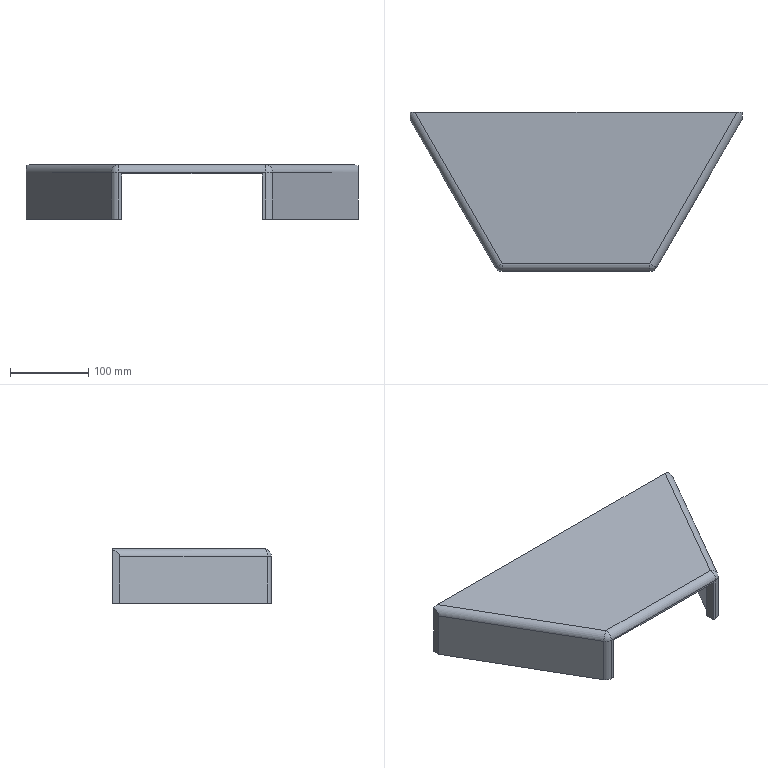Part | SolidWorks | features ICE 4, Fillet 2, Extrusion 1, Shell 1 | 1 solid | 25 faces | box 424 x 203 x 70 mm | volume 1081632 mm3 | plane 18 | cylinder 5 | sphere 2 | commonest cylinder face diameters 20 x5
STEP:
#1=CARTESIAN_POINT('',(90.,-95.5,58.));
#2=VERTEX_POINT('',#1);
#3=CARTESIAN_POINT('',(90.,-95.5,0.));
#4=VERTEX_POINT('',#3);
#5=CARTESIAN_POINT('',(90.,-95.5,70.));
#6=DIRECTION('',(0.,0.,-1.));
#7=VECTOR('',#6,1000.);
#8=LINE('',#5,#7);
#9=EDGE_CURVE('',#2,#4,#8,.T.);
#10=ORIENTED_EDGE('',*,*,#9,.F.);
#11=CARTESIAN_POINT('',(93.072,-95.5,58.));
#12=VERTEX_POINT('',#11);
#13=CARTESIAN_POINT('',(-93.072,-95.5,58.));
#14=DIRECTION('',(1.,0.,0.));
#15=VECTOR('',#14,1000.);
#16=LINE('',#13,#15);
#17=EDGE_CURVE('',#2,#12,#16,.T.);
#18=ORIENTED_EDGE('',*,*,#17,.T.);
#19=CARTESIAN_POINT('',(93.072,-95.5,0.));
#20=VERTEX_POINT('',#19);
#21=CARTESIAN_POINT('',(93.072,-95.5,70.));
#22=DIRECTION('',(0.,0.,-1.));
#23=VECTOR('',#22,1000.);
#24=LINE('',#21,#23);
#25=EDGE_CURVE('',#12,#20,#24,.T.);
#26=ORIENTED_EDGE('',*,*,#25,.T.);
#27=CARTESIAN_POINT('',(0.,-95.5,0.));
#28=DIRECTION('',(1.,0.,0.));
#29=VECTOR('',#28,1000.);
#30=LINE('',#27,#29);
#31=EDGE_CURVE('',#4,#20,#30,.T.);
#32=ORIENTED_EDGE('',*,*,#31,.F.);
#33=EDGE_LOOP('',(#10,#18,#26,#32));
#34=FACE_OUTER_BOUND('',#33,.T.);
#35=CARTESIAN_POINT('',(212.,-95.5,70.));
#36=DIRECTION('',(0.,1.,0.));
#37=DIRECTION('',(-1.,0.,0.));
#38=AXIS2_PLACEMENT_3D('',#35,#36,#37);
#39=PLANE('',#38);
#40=ADVANCED_FACE('',(#34),#39,.T.);
#41=CARTESIAN_POINT('',(212.,86.49,0.));
#42=VERTEX_POINT('',#41);
#43=CARTESIAN_POINT('',(102.887,-102.5,0.));
#44=VERTEX_POINT('',#43);
#45=CARTESIAN_POINT('',(121.549,-70.176,0.));
#46=DIRECTION('',(-0.5,-0.866,0.));
#47=VECTOR('',#46,1000.);
#48=LINE('',#45,#47);
#49=EDGE_CURVE('',#42,#44,#48,.T.);
#50=ORIENTED_EDGE('',*,*,#49,.T.);
#51=CARTESIAN_POINT('',(94.226,-107.5,0.));
#52=VERTEX_POINT('',#51);
#53=CARTESIAN_POINT('',(94.226,-97.5,0.));
#54=DIRECTION('',(0.,0.,-1.));
#55=DIRECTION('',(-1.,0.,0.));
#56=AXIS2_PLACEMENT_3D('',#53,#54,#55);
#57=CIRCLE('',#56,10.);
#58=EDGE_CURVE('',#44,#52,#57,.T.);
#59=ORIENTED_EDGE('',*,*,#58,.T.);
#60=CARTESIAN_POINT('',(90.,-107.5,0.));
#61=VERTEX_POINT('',#60);
#62=CARTESIAN_POINT('',(212.,-107.5,0.));
#63=DIRECTION('',(1.,0.,0.));
#64=VECTOR('',#63,1000.);
#65=LINE('',#62,#64);
#66=EDGE_CURVE('',#61,#52,#65,.T.);
#67=ORIENTED_EDGE('',*,*,#66,.F.);
#68=CARTESIAN_POINT('',(90.,0.,0.));
#69=DIRECTION('',(0.,-1.,0.));
#70=VECTOR('',#69,1000.);
#71=LINE('',#68,#70);
#72=EDGE_CURVE('',#4,#61,#71,.T.);
#73=ORIENTED_EDGE('',*,*,#72,.F.);
#74=ORIENTED_EDGE('',*,*,#31,.T.);
#75=CARTESIAN_POINT('',(200.,89.705,0.));
#76=VERTEX_POINT('',#75);
#77=CARTESIAN_POINT('',(111.157,-64.176,0.));
#78=DIRECTION('',(-0.5,-0.866,0.));
#79=VECTOR('',#78,1000.);
#80=LINE('',#77,#79);
#81=EDGE_CURVE('',#76,#20,#80,.T.);
#82=ORIENTED_EDGE('',*,*,#81,.F.);
#83=CARTESIAN_POINT('',(200.,95.5,0.));
#84=VERTEX_POINT('',#83);
#85=CARTESIAN_POINT('',(200.,0.,0.));
#86=DIRECTION('',(0.,1.,0.));
#87=VECTOR('',#86,1000.);
#88=LINE('',#85,#87);
#89=EDGE_CURVE('',#76,#84,#88,.T.);
#90=ORIENTED_EDGE('',*,*,#89,.T.);
#91=CARTESIAN_POINT('',(212.,95.5,0.));
#92=VERTEX_POINT('',#91);
#93=CARTESIAN_POINT('',(-212.,95.5,0.));
#94=DIRECTION('',(-1.,0.,0.));
#95=VECTOR('',#94,1000.);
#96=LINE('',#93,#95);
#97=EDGE_CURVE('',#92,#84,#96,.T.);
#98=ORIENTED_EDGE('',*,*,#97,.F.);
#99=CARTESIAN_POINT('',(212.,107.5,0.));
#100=DIRECTION('',(0.,1.,0.));
#101=VECTOR('',#100,1000.);
#102=LINE('',#99,#101);
#103=EDGE_CURVE('',#42,#92,#102,.T.);
#104=ORIENTED_EDGE('',*,*,#103,.F.);
#105=EDGE_LOOP('',(#50,#59,#67,#73,#74,#82,#90,#98,#104));
#106=FACE_OUTER_BOUND('',#105,.T.);
#107=CARTESIAN_POINT('',(0.,0.,0.));
#108=DIRECTION('',(0.,0.,-1.));
#109=DIRECTION('',(-1.,0.,0.));
#110=AXIS2_PLACEMENT_3D('',#107,#108,#109);
#111=PLANE('',#110);
#112=ADVANCED_FACE('',(#106),#111,.T.);
#113=CARTESIAN_POINT('',(-200.,95.5,58.));
#114=VERTEX_POINT('',#113);
#115=CARTESIAN_POINT('',(-200.,95.5,0.));
#116=VERTEX_POINT('',#115);
#117=CARTESIAN_POINT('',(-200.,95.5,70.));
#118=DIRECTION('',(0.,0.,-1.));
#119=VECTOR('',#118,1000.);
#120=LINE('',#117,#119);
#121=EDGE_CURVE('',#114,#116,#120,.T.);
#122=ORIENTED_EDGE('',*,*,#121,.F.);
#123=CARTESIAN_POINT('',(-200.,89.705,58.));
#124=VERTEX_POINT('',#123);
#125=CARTESIAN_POINT('',(-200.,89.705,58.));
#126=DIRECTION('',(0.,-1.,0.));
#127=VECTOR('',#126,1000.);
#128=LINE('',#125,#127);
#129=EDGE_CURVE('',#114,#124,#128,.T.);
#130=ORIENTED_EDGE('',*,*,#129,.T.);
#131=CARTESIAN_POINT('',(-200.,89.705,0.));
#132=VERTEX_POINT('',#131);
#133=CARTESIAN_POINT('',(-200.,89.705,70.));
#134=DIRECTION('',(0.,0.,-1.));
#135=VECTOR('',#134,1000.);
#136=LINE('',#133,#135);
#137=EDGE_CURVE('',#124,#132,#136,.T.);
#138=ORIENTED_EDGE('',*,*,#137,.T.);
#139=CARTESIAN_POINT('',(-200.,0.,0.));
#140=DIRECTION('',(0.,-1.,0.));
#141=VECTOR('',#140,1000.);
#142=LINE('',#139,#141);
#143=EDGE_CURVE('',#116,#132,#142,.T.);
#144=ORIENTED_EDGE('',*,*,#143,.F.);
#145=EDGE_LOOP('',(#122,#130,#138,#144));
#146=FACE_OUTER_BOUND('',#145,.T.);
#147=CARTESIAN_POINT('',(-200.,107.5,70.));
#148=DIRECTION('',(1.,0.,0.));
#149=DIRECTION('',(0.,1.,0.));
#150=AXIS2_PLACEMENT_3D('',#147,#148,#149);
#151=PLANE('',#150);
#152=ADVANCED_FACE('',(#146),#151,.T.);
#153=CARTESIAN_POINT('',(-90.,-95.5,0.));
#154=VERTEX_POINT('',#153);
#155=CARTESIAN_POINT('',(-90.,-95.5,58.));
#156=VERTEX_POINT('',#155);
#157=CARTESIAN_POINT('',(-90.,-95.5,70.));
#158=DIRECTION('',(0.,0.,1.));
#159=VECTOR('',#158,1000.);
#160=LINE('',#157,#159);
#161=EDGE_CURVE('',#154,#156,#160,.T.);
#162=ORIENTED_EDGE('',*,*,#161,.F.);
#163=CARTESIAN_POINT('',(-93.072,-95.5,0.));
#164=VERTEX_POINT('',#163);
#165=CARTESIAN_POINT('',(0.,-95.5,0.));
#166=DIRECTION('',(1.,0.,0.));
#167=VECTOR('',#166,1000.);
#168=LINE('',#165,#167);
#169=EDGE_CURVE('',#164,#154,#168,.T.);
#170=ORIENTED_EDGE('',*,*,#169,.F.);
#171=CARTESIAN_POINT('',(-93.072,-95.5,58.));
#172=VERTEX_POINT('',#171);
#173=CARTESIAN_POINT('',(-93.072,-95.5,70.));
#174=DIRECTION('',(0.,0.,-1.));
#175=VECTOR('',#174,1000.);
#176=LINE('',#173,#175);
#177=EDGE_CURVE('',#172,#164,#176,.T.);
#178=ORIENTED_EDGE('',*,*,#177,.F.);
#179=CARTESIAN_POINT('',(-93.072,-95.5,58.));
#180=DIRECTION('',(1.,0.,0.));
#181=VECTOR('',#180,1000.);
#182=LINE('',#179,#181);
#183=EDGE_CURVE('',#172,#156,#182,.T.);
#184=ORIENTED_EDGE('',*,*,#183,.T.);
#185=EDGE_LOOP('',(#162,#170,#178,#184));
#186=FACE_OUTER_BOUND('',#185,.T.);
#187=CARTESIAN_POINT('',(212.,-95.5,70.));
#188=DIRECTION('',(0.,1.,0.));
#189=DIRECTION('',(-1.,0.,0.));
#190=AXIS2_PLACEMENT_3D('',#187,#188,#189);
#191=PLANE('',#190);
#192=ADVANCED_FACE('',(#186),#191,.T.);
#193=CARTESIAN_POINT('',(200.,89.705,58.));
#194=VERTEX_POINT('',#193);
#195=CARTESIAN_POINT('',(200.,89.705,70.));
#196=DIRECTION('',(0.,0.,1.));
#197=VECTOR('',#196,1000.);
#198=LINE('',#195,#197);
#199=EDGE_CURVE('',#76,#194,#198,.T.);
#200=ORIENTED_EDGE('',*,*,#199,.T.);
#201=CARTESIAN_POINT('',(200.,95.5,58.));
#202=VERTEX_POINT('',#201);
#203=CARTESIAN_POINT('',(200.,89.705,58.));
#204=DIRECTION('',(0.,1.,0.));
#205=VECTOR('',#204,1000.);
#206=LINE('',#203,#205);
#207=EDGE_CURVE('',#194,#202,#206,.T.);
#208=ORIENTED_EDGE('',*,*,#207,.T.);
#209=CARTESIAN_POINT('',(200.,95.5,70.));
#210=DIRECTION('',(0.,0.,-1.));
#211=VECTOR('',#210,1000.);
#212=LINE('',#209,#211);
#213=EDGE_CURVE('',#202,#84,#212,.T.);
#214=ORIENTED_EDGE('',*,*,#213,.T.);
#215=ORIENTED_EDGE('',*,*,#89,.F.);
#216=EDGE_LOOP('',(#200,#208,#214,#215));
#217=FACE_OUTER_BOUND('',#216,.T.);
#218=CARTESIAN_POINT('',(200.,107.5,70.));
#219=DIRECTION('',(-1.,0.,0.));
#220=DIRECTION('',(0.,-1.,0.));
#221=AXIS2_PLACEMENT_3D('',#218,#219,#220);
#222=PLANE('',#221);
#223=ADVANCED_FACE('',(#217),#222,.T.);
#224=CARTESIAN_POINT('',(200.,89.705,58.));
#225=DIRECTION('',(0.5,0.866,0.));
#226=VECTOR('',#225,1000.);
#227=LINE('',#224,#226);
#228=EDGE_CURVE('',#12,#194,#227,.T.);
#229=ORIENTED_EDGE('',*,*,#228,.T.);
#230=ORIENTED_EDGE('',*,*,#199,.F.);
#231=ORIENTED_EDGE('',*,*,#81,.T.);
#232=ORIENTED_EDGE('',*,*,#25,.F.);
#233=EDGE_LOOP('',(#229,#230,#231,#232));
#234=FACE_OUTER_BOUND('',#233,.T.);
#235=CARTESIAN_POINT('',(89.608,-101.5,70.));
#236=DIRECTION('',(0.866,-0.5,0.));
#237=DIRECTION('',(0.5,0.866,0.));
#238=AXIS2_PLACEMENT_3D('',#235,#236,#237);
#239=PLANE('',#238);
#240=ADVANCED_FACE('',(#234),#239,.F.);
#241=CARTESIAN_POINT('',(-93.072,-95.5,58.));
#242=DIRECTION('',(0.5,-0.866,0.));
#243=VECTOR('',#242,1000.);
#244=LINE('',#241,#243);
#245=EDGE_CURVE('',#124,#172,#244,.T.);
#246=ORIENTED_EDGE('',*,*,#245,.T.);
#247=ORIENTED_EDGE('',*,*,#177,.T.);
#248=CARTESIAN_POINT('',(-111.157,-64.176,0.));
#249=DIRECTION('',(-0.5,0.866,0.));
#250=VECTOR('',#249,1000.);
#251=LINE('',#248,#250);
#252=EDGE_CURVE('',#164,#132,#251,.T.);
#253=ORIENTED_EDGE('',*,*,#252,.T.);
#254=ORIENTED_EDGE('',*,*,#137,.F.);
#255=EDGE_LOOP('',(#246,#247,#253,#254));
#256=FACE_OUTER_BOUND('',#255,.T.);
#257=CARTESIAN_POINT('',(-213.738,113.5,70.));
#258=DIRECTION('',(-0.866,-0.5,0.));
#259=DIRECTION('',(0.5,-0.866,0.));
#260=AXIS2_PLACEMENT_3D('',#257,#258,#259);
#261=PLANE('',#260);
#262=ADVANCED_FACE('',(#256),#261,.F.);
#263=CARTESIAN_POINT('',(-94.226,-107.5,0.));
#264=VERTEX_POINT('',#263);
#265=CARTESIAN_POINT('',(-90.,-107.5,0.));
#266=VERTEX_POINT('',#265);
#267=CARTESIAN_POINT('',(212.,-107.5,0.));
#268=DIRECTION('',(1.,0.,0.));
#269=VECTOR('',#268,1000.);
#270=LINE('',#267,#269);
#271=EDGE_CURVE('',#264,#266,#270,.T.);
#272=ORIENTED_EDGE('',*,*,#271,.F.);
#273=CARTESIAN_POINT('',(-102.887,-102.5,0.));
#274=VERTEX_POINT('',#273);
#275=CARTESIAN_POINT('',(-94.226,-97.5,0.));
#276=DIRECTION('',(0.,0.,-1.));
#277=DIRECTION('',(-1.,0.,0.));
#278=AXIS2_PLACEMENT_3D('',#275,#276,#277);
#279=CIRCLE('',#278,10.);
#280=EDGE_CURVE('',#264,#274,#279,.T.);
#281=ORIENTED_EDGE('',*,*,#280,.T.);
#282=CARTESIAN_POINT('',(-212.,86.49,0.));
#283=VERTEX_POINT('',#282);
#284=CARTESIAN_POINT('',(-224.13,107.5,0.));
#285=DIRECTION('',(-0.5,0.866,0.));
#286=VECTOR('',#285,1000.);
#287=LINE('',#284,#286);
#288=EDGE_CURVE('',#274,#283,#287,.T.);
#289=ORIENTED_EDGE('',*,*,#288,.T.);
#290=CARTESIAN_POINT('',(-212.,95.5,0.));
#291=VERTEX_POINT('',#290);
#292=CARTESIAN_POINT('',(-212.,107.5,0.));
#293=DIRECTION('',(0.,-1.,0.));
#294=VECTOR('',#293,1000.);
#295=LINE('',#292,#294);
#296=EDGE_CURVE('',#291,#283,#295,.T.);
#297=ORIENTED_EDGE('',*,*,#296,.F.);
#298=CARTESIAN_POINT('',(-212.,95.5,0.));
#299=DIRECTION('',(-1.,0.,0.));
#300=VECTOR('',#299,1000.);
#301=LINE('',#298,#300);
#302=EDGE_CURVE('',#116,#291,#301,.T.);
#303=ORIENTED_EDGE('',*,*,#302,.F.);
#304=ORIENTED_EDGE('',*,*,#143,.T.);
#305=ORIENTED_EDGE('',*,*,#252,.F.);
#306=ORIENTED_EDGE('',*,*,#169,.T.);
#307=CARTESIAN_POINT('',(-90.,0.,0.));
#308=DIRECTION('',(0.,1.,0.));
#309=VECTOR('',#308,1000.);
#310=LINE('',#307,#309);
#311=EDGE_CURVE('',#266,#154,#310,.T.);
#312=ORIENTED_EDGE('',*,*,#311,.F.);
#313=EDGE_LOOP('',(#272,#281,#289,#297,#303,#304,#305,#306,#312));
#314=FACE_OUTER_BOUND('',#313,.T.);
#315=CARTESIAN_POINT('',(0.,0.,0.));
#316=DIRECTION('',(0.,0.,-1.));
#317=DIRECTION('',(-1.,0.,0.));
#318=AXIS2_PLACEMENT_3D('',#315,#316,#317);
#319=PLANE('',#318);
#320=ADVANCED_FACE('',(#314),#319,.T.);
#321=CARTESIAN_POINT('',(-212.,86.49,60.));
#322=VERTEX_POINT('',#321);
#323=CARTESIAN_POINT('',(-212.,86.49,70.));
#324=DIRECTION('',(0.,0.,-1.));
#325=VECTOR('',#324,1000.);
#326=LINE('',#323,#325);
#327=EDGE_CURVE('',#322,#283,#326,.T.);
#328=ORIENTED_EDGE('',*,*,#327,.F.);
#329=CARTESIAN_POINT('',(-212.,95.5,68.355));
#330=VERTEX_POINT('',#329);
#331=CARTESIAN_POINT('',(-212.,86.49,60.));
#332=CARTESIAN_POINT('',(-212.,86.49,63.439));
#333=CARTESIAN_POINT('',(-212.,89.754,66.466));
#334=CARTESIAN_POINT('',(-212.,95.5,68.355));
#335=(BOUNDED_CURVE()B_SPLINE_CURVE(3,(#331,#332,#333,#334),.UNSPECIFIED.,.F.,.F.)B_SPLINE_CURVE_WITH_KNOTS((4,4),(0.,0.989),.UNSPECIFIED.)CURVE()GEOMETRIC_REPRESENTATION_ITEM()RATIONAL_B_SPLINE_CURVE((1.,0.9201,0.9201,1.))REPRESENTATION_ITEM(''));
#336=EDGE_CURVE('',#322,#330,#335,.T.);
#337=ORIENTED_EDGE('',*,*,#336,.T.);
#338=CARTESIAN_POINT('',(-212.,95.5,70.));
#339=DIRECTION('',(0.,0.,-1.));
#340=VECTOR('',#339,1000.);
#341=LINE('',#338,#340);
#342=EDGE_CURVE('',#330,#291,#341,.T.);
#343=ORIENTED_EDGE('',*,*,#342,.T.);
#344=ORIENTED_EDGE('',*,*,#296,.T.);
#345=EDGE_LOOP('',(#328,#337,#343,#344));
#346=FACE_OUTER_BOUND('',#345,.T.);
#347=CARTESIAN_POINT('',(-212.,107.5,70.));
#348=DIRECTION('',(1.,0.,0.));
#349=DIRECTION('',(0.,1.,0.));
#350=AXIS2_PLACEMENT_3D('',#347,#348,#349);
#351=PLANE('',#350);
#352=ADVANCED_FACE('',(#346),#351,.F.);
#353=CARTESIAN_POINT('',(94.226,-107.5,60.));
#354=VERTEX_POINT('',#353);
#355=CARTESIAN_POINT('',(-94.226,-107.5,60.));
#356=VERTEX_POINT('',#355);
#357=CARTESIAN_POINT('',(212.,-107.5,60.));
#358=DIRECTION('',(-1.,0.,0.));
#359=VECTOR('',#358,1000.);
#360=LINE('',#357,#359);
#361=EDGE_CURVE('',#354,#356,#360,.T.);
#362=ORIENTED_EDGE('',*,*,#361,.T.);
#363=CARTESIAN_POINT('',(-94.226,-107.5,0.));
#364=DIRECTION('',(0.,0.,-1.));
#365=VECTOR('',#364,1000.);
#366=LINE('',#363,#365);
#367=EDGE_CURVE('',#356,#264,#366,.T.);
#368=ORIENTED_EDGE('',*,*,#367,.T.);
#369=ORIENTED_EDGE('',*,*,#271,.T.);
#370=CARTESIAN_POINT('',(-90.,-107.5,58.));
#371=VERTEX_POINT('',#370);
#372=CARTESIAN_POINT('',(-90.,-107.5,-74.019));
#373=DIRECTION('',(0.,0.,-1.));
#374=VECTOR('',#373,1000.);
#375=LINE('',#372,#374);
#376=EDGE_CURVE('',#371,#266,#375,.T.);
#377=ORIENTED_EDGE('',*,*,#376,.F.);
#378=CARTESIAN_POINT('',(90.,-107.5,58.));
#379=VERTEX_POINT('',#378);
#380=CARTESIAN_POINT('',(-90.,-107.5,58.));
#381=DIRECTION('',(-1.,0.,0.));
#382=VECTOR('',#381,1000.);
#383=LINE('',#380,#382);
#384=EDGE_CURVE('',#379,#371,#383,.T.);
#385=ORIENTED_EDGE('',*,*,#384,.F.);
#386=CARTESIAN_POINT('',(90.,-107.5,-74.019));
#387=DIRECTION('',(0.,0.,1.));
#388=VECTOR('',#387,1000.);
#389=LINE('',#386,#388);
#390=EDGE_CURVE('',#61,#379,#389,.T.);
#391=ORIENTED_EDGE('',*,*,#390,.F.);
#392=ORIENTED_EDGE('',*,*,#66,.T.);
#393=CARTESIAN_POINT('',(94.226,-107.5,70.));
#394=DIRECTION('',(0.,0.,1.));
#395=VECTOR('',#394,1000.);
#396=LINE('',#393,#395);
#397=EDGE_CURVE('',#52,#354,#396,.T.);
#398=ORIENTED_EDGE('',*,*,#397,.T.);
#399=EDGE_LOOP('',(#362,#368,#369,#377,#385,#391,#392,#398));
#400=FACE_OUTER_BOUND('',#399,.T.);
#401=CARTESIAN_POINT('',(212.,-107.5,70.));
#402=DIRECTION('',(0.,1.,0.));
#403=DIRECTION('',(-1.,0.,0.));
#404=AXIS2_PLACEMENT_3D('',#401,#402,#403);
#405=PLANE('',#404);
#406=ADVANCED_FACE('',(#400),#405,.F.);
#407=CARTESIAN_POINT('',(212.,95.5,68.355));
#408=VERTEX_POINT('',#407);
#409=CARTESIAN_POINT('',(212.,95.5,70.));
#410=DIRECTION('',(0.,0.,1.));
#411=VECTOR('',#410,1000.);
#412=LINE('',#409,#411);
#413=EDGE_CURVE('',#92,#408,#412,.T.);
#414=ORIENTED_EDGE('',*,*,#413,.T.);
#415=CARTESIAN_POINT('',(212.,86.49,60.));
#416=VERTEX_POINT('',#415);
#417=CARTESIAN_POINT('',(212.,95.5,68.355));
#418=CARTESIAN_POINT('',(212.,89.754,66.466));
#419=CARTESIAN_POINT('',(212.,86.49,63.439));
#420=CARTESIAN_POINT('',(212.,86.49,60.));
#421=(BOUNDED_CURVE()B_SPLINE_CURVE(3,(#417,#418,#419,#420),.UNSPECIFIED.,.F.,.T.)B_SPLINE_CURVE_WITH_KNOTS((4,4),(2.153,3.142),.UNSPECIFIED.)CURVE()GEOMETRIC_REPRESENTATION_ITEM()RATIONAL_B_SPLINE_CURVE((1.,0.9201,0.9201,1.))REPRESENTATION_ITEM(''));
#422=EDGE_CURVE('',#408,#416,#421,.T.);
#423=ORIENTED_EDGE('',*,*,#422,.T.);
#424=CARTESIAN_POINT('',(212.,86.49,70.));
#425=DIRECTION('',(0.,0.,1.));
#426=VECTOR('',#425,1000.);
#427=LINE('',#424,#426);
#428=EDGE_CURVE('',#42,#416,#427,.T.);
#429=ORIENTED_EDGE('',*,*,#428,.F.);
#430=ORIENTED_EDGE('',*,*,#103,.T.);
#431=EDGE_LOOP('',(#414,#423,#429,#430));
#432=FACE_OUTER_BOUND('',#431,.T.);
#433=CARTESIAN_POINT('',(212.,107.5,70.));
#434=DIRECTION('',(-1.,0.,0.));
#435=DIRECTION('',(0.,-1.,0.));
#436=AXIS2_PLACEMENT_3D('',#433,#434,#435);
#437=PLANE('',#436);
#438=ADVANCED_FACE('',(#432),#437,.F.);
#439=CARTESIAN_POINT('',(-94.226,-97.5,70.));
#440=VERTEX_POINT('',#439);
#441=CARTESIAN_POINT('',(94.226,-97.5,70.));
#442=VERTEX_POINT('',#441);
#443=CARTESIAN_POINT('',(0.,-97.5,70.));
#444=DIRECTION('',(1.,0.,0.));
#445=VECTOR('',#444,1000.);
#446=LINE('',#443,#445);
#447=EDGE_CURVE('',#440,#442,#446,.T.);
#448=ORIENTED_EDGE('',*,*,#447,.T.);
#449=CARTESIAN_POINT('',(205.655,95.5,70.));
#450=VERTEX_POINT('',#449);
#451=CARTESIAN_POINT('',(203.34,91.49,70.));
#452=DIRECTION('',(0.5,0.866,0.));
#453=VECTOR('',#452,1000.);
#454=LINE('',#451,#453);
#455=EDGE_CURVE('',#442,#450,#454,.T.);
#456=ORIENTED_EDGE('',*,*,#455,.T.);
#457=CARTESIAN_POINT('',(-205.655,95.5,70.));
#458=VERTEX_POINT('',#457);
#459=CARTESIAN_POINT('',(-212.,95.5,70.));
#460=DIRECTION('',(-1.,0.,0.));
#461=VECTOR('',#460,1000.);
#462=LINE('',#459,#461);
#463=EDGE_CURVE('',#450,#458,#462,.T.);
#464=ORIENTED_EDGE('',*,*,#463,.T.);
#465=CARTESIAN_POINT('',(-97.113,-92.5,70.));
#466=DIRECTION('',(0.5,-0.866,0.));
#467=VECTOR('',#466,1000.);
#468=LINE('',#465,#467);
#469=EDGE_CURVE('',#458,#440,#468,.T.);
#470=ORIENTED_EDGE('',*,*,#469,.T.);
#471=EDGE_LOOP('',(#448,#456,#464,#470));
#472=FACE_OUTER_BOUND('',#471,.T.);
#473=CARTESIAN_POINT('',(0.,0.,70.));
#474=DIRECTION('',(0.,0.,-1.));
#475=DIRECTION('',(-1.,0.,0.));
#476=AXIS2_PLACEMENT_3D('',#473,#474,#475);
#477=PLANE('',#476);
#478=ADVANCED_FACE('',(#472),#477,.F.);
#479=ORIENTED_EDGE('',*,*,#428,.T.);
#480=CARTESIAN_POINT('',(102.887,-102.5,60.));
#481=VERTEX_POINT('',#480);
#482=CARTESIAN_POINT('',(105.774,-97.5,60.));
#483=DIRECTION('',(-0.5,-0.866,0.));
#484=VECTOR('',#483,1000.);
#485=LINE('',#482,#484);
#486=EDGE_CURVE('',#416,#481,#485,.T.);
#487=ORIENTED_EDGE('',*,*,#486,.T.);
#488=CARTESIAN_POINT('',(102.887,-102.5,0.));
#489=DIRECTION('',(0.,0.,-1.));
#490=VECTOR('',#489,1000.);
#491=LINE('',#488,#490);
#492=EDGE_CURVE('',#481,#44,#491,.T.);
#493=ORIENTED_EDGE('',*,*,#492,.T.);
#494=ORIENTED_EDGE('',*,*,#49,.F.);
#495=EDGE_LOOP('',(#479,#487,#493,#494));
#496=FACE_OUTER_BOUND('',#495,.T.);
#497=CARTESIAN_POINT('',(100.,-107.5,70.));
#498=DIRECTION('',(0.866,-0.5,0.));
#499=DIRECTION('',(0.5,0.866,0.));
#500=AXIS2_PLACEMENT_3D('',#497,#498,#499);
#501=PLANE('',#500);
#502=ADVANCED_FACE('',(#496),#501,.T.);
#503=CARTESIAN_POINT('',(-102.887,-102.5,60.));
#504=VERTEX_POINT('',#503);
#505=CARTESIAN_POINT('',(-102.887,-102.5,70.));
#506=DIRECTION('',(0.,0.,1.));
#507=VECTOR('',#506,1000.);
#508=LINE('',#505,#507);
#509=EDGE_CURVE('',#274,#504,#508,.T.);
#510=ORIENTED_EDGE('',*,*,#509,.T.);
#511=CARTESIAN_POINT('',(-212.,86.49,60.));
#512=DIRECTION('',(-0.5,0.866,0.));
#513=VECTOR('',#512,1000.);
#514=LINE('',#511,#513);
#515=EDGE_CURVE('',#504,#322,#514,.T.);
#516=ORIENTED_EDGE('',*,*,#515,.T.);
#517=ORIENTED_EDGE('',*,*,#327,.T.);
#518=ORIENTED_EDGE('',*,*,#288,.F.);
#519=EDGE_LOOP('',(#510,#516,#517,#518));
#520=FACE_OUTER_BOUND('',#519,.T.);
#521=CARTESIAN_POINT('',(-224.13,107.5,70.));
#522=DIRECTION('',(-0.866,-0.5,0.));
#523=DIRECTION('',(0.5,-0.866,0.));
#524=AXIS2_PLACEMENT_3D('',#521,#522,#523);
#525=PLANE('',#524);
#526=ADVANCED_FACE('',(#520),#525,.T.);
#527=ORIENTED_EDGE('',*,*,#17,.F.);
#528=CARTESIAN_POINT('',(90.,-37.5,58.));
#529=DIRECTION('',(0.,-1.,0.));
#530=VECTOR('',#529,1000.);
#531=LINE('',#528,#530);
#532=EDGE_CURVE('',#2,#379,#531,.T.);
#533=ORIENTED_EDGE('',*,*,#532,.T.);
#534=ORIENTED_EDGE('',*,*,#384,.T.);
#535=CARTESIAN_POINT('',(-90.,-37.5,58.));
#536=DIRECTION('',(0.,-1.,0.));
#537=VECTOR('',#536,1000.);
#538=LINE('',#535,#537);
#539=EDGE_CURVE('',#156,#371,#538,.T.);
#540=ORIENTED_EDGE('',*,*,#539,.F.);
#541=ORIENTED_EDGE('',*,*,#183,.F.);
#542=ORIENTED_EDGE('',*,*,#245,.F.);
#543=ORIENTED_EDGE('',*,*,#129,.F.);
#544=CARTESIAN_POINT('',(200.,95.5,58.));
#545=DIRECTION('',(-1.,0.,0.));
#546=VECTOR('',#545,1000.);
#547=LINE('',#544,#546);
#548=EDGE_CURVE('',#202,#114,#547,.T.);
#549=ORIENTED_EDGE('',*,*,#548,.F.);
#550=ORIENTED_EDGE('',*,*,#207,.F.);
#551=ORIENTED_EDGE('',*,*,#228,.F.);
#552=EDGE_LOOP('',(#527,#533,#534,#540,#541,#542,#543,#549,#550,#551));
#553=FACE_OUTER_BOUND('',#552,.T.);
#554=CARTESIAN_POINT('',(0.,0.,58.));
#555=DIRECTION('',(0.,0.,1.));
#556=DIRECTION('',(1.,0.,0.));
#557=AXIS2_PLACEMENT_3D('',#554,#555,#556);
#558=PLANE('',#557);
#559=ADVANCED_FACE('',(#553),#558,.F.);
#560=ORIENTED_EDGE('',*,*,#463,.F.);
#561=CARTESIAN_POINT('',(205.655,95.5,70.));
#562=CARTESIAN_POINT('',(207.926,95.5,70.));
#563=CARTESIAN_POINT('',(210.102,95.5,69.436));
#564=CARTESIAN_POINT('',(212.,95.5,68.355));
#565=(BOUNDED_CURVE()B_SPLINE_CURVE(3,(#561,#562,#563,#564),.UNSPECIFIED.,.F.,.T.)B_SPLINE_CURVE_WITH_KNOTS((4,4),(4.712,5.294),.UNSPECIFIED.)CURVE()GEOMETRIC_REPRESENTATION_ITEM()RATIONAL_B_SPLINE_CURVE((1.,0.972,0.972,1.))REPRESENTATION_ITEM(''));
#566=EDGE_CURVE('',#450,#408,#565,.T.);
#567=ORIENTED_EDGE('',*,*,#566,.T.);
#568=ORIENTED_EDGE('',*,*,#413,.F.);
#569=ORIENTED_EDGE('',*,*,#97,.T.);
#570=ORIENTED_EDGE('',*,*,#213,.F.);
#571=ORIENTED_EDGE('',*,*,#548,.T.);
#572=ORIENTED_EDGE('',*,*,#121,.T.);
#573=ORIENTED_EDGE('',*,*,#302,.T.);
#574=ORIENTED_EDGE('',*,*,#342,.F.);
#575=CARTESIAN_POINT('',(-212.,95.5,68.355));
#576=CARTESIAN_POINT('',(-210.102,95.5,69.436));
#577=CARTESIAN_POINT('',(-207.926,95.5,70.));
#578=CARTESIAN_POINT('',(-205.655,95.5,70.));
#579=(BOUNDED_CURVE()B_SPLINE_CURVE(3,(#575,#576,#577,#578),.UNSPECIFIED.,.F.,.F.)B_SPLINE_CURVE_WITH_KNOTS((4,4),(4.131,4.712),.UNSPECIFIED.)CURVE()GEOMETRIC_REPRESENTATION_ITEM()RATIONAL_B_SPLINE_CURVE((1.,0.972,0.972,1.))REPRESENTATION_ITEM(''));
#580=EDGE_CURVE('',#330,#458,#579,.T.);
#581=ORIENTED_EDGE('',*,*,#580,.T.);
#582=EDGE_LOOP('',(#560,#567,#568,#569,#570,#571,#572,#573,#574,#581));
#583=FACE_OUTER_BOUND('',#582,.T.);
#584=CARTESIAN_POINT('',(-212.,95.5,70.));
#585=DIRECTION('',(0.,-1.,0.));
#586=DIRECTION('',(1.,0.,0.));
#587=AXIS2_PLACEMENT_3D('',#584,#585,#586);
#588=PLANE('',#587);
#589=ADVANCED_FACE('',(#583),#588,.F.);
#590=ORIENTED_EDGE('',*,*,#9,.T.);
#591=ORIENTED_EDGE('',*,*,#72,.T.);
#592=ORIENTED_EDGE('',*,*,#390,.T.);
#593=ORIENTED_EDGE('',*,*,#532,.F.);
#594=EDGE_LOOP('',(#590,#591,#592,#593));
#595=FACE_OUTER_BOUND('',#594,.T.);
#596=CARTESIAN_POINT('',(90.,-37.5,-74.019));
#597=DIRECTION('',(1.,0.,0.));
#598=DIRECTION('',(0.,1.,0.));
#599=AXIS2_PLACEMENT_3D('',#596,#597,#598);
#600=PLANE('',#599);
#601=ADVANCED_FACE('',(#595),#600,.F.);
#602=ORIENTED_EDGE('',*,*,#161,.T.);
#603=ORIENTED_EDGE('',*,*,#539,.T.);
#604=ORIENTED_EDGE('',*,*,#376,.T.);
#605=ORIENTED_EDGE('',*,*,#311,.T.);
#606=EDGE_LOOP('',(#602,#603,#604,#605));
#607=FACE_OUTER_BOUND('',#606,.T.);
#608=CARTESIAN_POINT('',(-90.,-37.5,-74.019));
#609=DIRECTION('',(-1.,0.,0.));
#610=DIRECTION('',(0.,-1.,0.));
#611=AXIS2_PLACEMENT_3D('',#608,#609,#610);
#612=PLANE('',#611);
#613=ADVANCED_FACE('',(#607),#612,.F.);
#614=ORIENTED_EDGE('',*,*,#492,.F.);
#615=CARTESIAN_POINT('',(94.226,-97.5,60.));
#616=DIRECTION('',(0.,0.,-1.));
#617=DIRECTION('',(1.,0.,0.));
#618=AXIS2_PLACEMENT_3D('',#615,#616,#617);
#619=CIRCLE('',#618,10.);
#620=EDGE_CURVE('',#481,#354,#619,.T.);
#621=ORIENTED_EDGE('',*,*,#620,.T.);
#622=ORIENTED_EDGE('',*,*,#397,.F.);
#623=ORIENTED_EDGE('',*,*,#58,.F.);
#624=EDGE_LOOP('',(#614,#621,#622,#623));
#625=FACE_OUTER_BOUND('',#624,.T.);
#626=CARTESIAN_POINT('',(94.226,-97.5,70.));
#627=DIRECTION('',(0.,0.,1.));
#628=DIRECTION('',(1.,0.,0.));
#629=AXIS2_PLACEMENT_3D('',#626,#627,#628);
#630=CYLINDRICAL_SURFACE('',#629,10.);
#631=ADVANCED_FACE('',(#625),#630,.T.);
#632=ORIENTED_EDGE('',*,*,#361,.F.);
#633=CARTESIAN_POINT('',(94.226,-97.5,60.));
#634=DIRECTION('',(-1.,0.,0.));
#635=DIRECTION('',(0.,1.,0.));
#636=AXIS2_PLACEMENT_3D('',#633,#634,#635);
#637=CIRCLE('',#636,10.);
#638=EDGE_CURVE('',#354,#442,#637,.T.);
#639=ORIENTED_EDGE('',*,*,#638,.T.);
#640=ORIENTED_EDGE('',*,*,#447,.F.);
#641=CARTESIAN_POINT('',(-94.226,-97.5,60.));
#642=DIRECTION('',(1.,0.,0.));
#643=DIRECTION('',(0.,1.,0.));
#644=AXIS2_PLACEMENT_3D('',#641,#642,#643);
#645=CIRCLE('',#644,10.);
#646=EDGE_CURVE('',#440,#356,#645,.T.);
#647=ORIENTED_EDGE('',*,*,#646,.T.);
#648=EDGE_LOOP('',(#632,#639,#640,#647));
#649=FACE_OUTER_BOUND('',#648,.T.);
#650=CARTESIAN_POINT('',(0.,-97.5,60.));
#651=DIRECTION('',(1.,0.,0.));
#652=DIRECTION('',(0.,1.,0.));
#653=AXIS2_PLACEMENT_3D('',#650,#651,#652);
#654=CYLINDRICAL_SURFACE('',#653,10.);
#655=ADVANCED_FACE('',(#649),#654,.T.);
#656=ORIENTED_EDGE('',*,*,#367,.F.);
#657=CARTESIAN_POINT('',(-94.226,-97.5,60.));
#658=DIRECTION('',(0.,0.,-1.));
#659=DIRECTION('',(1.,0.,0.));
#660=AXIS2_PLACEMENT_3D('',#657,#658,#659);
#661=CIRCLE('',#660,10.);
#662=EDGE_CURVE('',#356,#504,#661,.T.);
#663=ORIENTED_EDGE('',*,*,#662,.T.);
#664=ORIENTED_EDGE('',*,*,#509,.F.);
#665=ORIENTED_EDGE('',*,*,#280,.F.);
#666=EDGE_LOOP('',(#656,#663,#664,#665));
#667=FACE_OUTER_BOUND('',#666,.T.);
#668=CARTESIAN_POINT('',(-94.226,-97.5,70.));
#669=DIRECTION('',(0.,0.,1.));
#670=DIRECTION('',(1.,0.,0.));
#671=AXIS2_PLACEMENT_3D('',#668,#669,#670);
#672=CYLINDRICAL_SURFACE('',#671,10.);
#673=ADVANCED_FACE('',(#667),#672,.T.);
#674=CARTESIAN_POINT('',(94.226,-97.5,60.));
#675=DIRECTION('',(-0.5,-0.866,0.));
#676=DIRECTION('',(0.866,-0.5,0.));
#677=AXIS2_PLACEMENT_3D('',#674,#675,#676);
#678=CIRCLE('',#677,10.);
#679=EDGE_CURVE('',#481,#442,#678,.T.);
#680=ORIENTED_EDGE('',*,*,#679,.F.);
#681=ORIENTED_EDGE('',*,*,#486,.F.);
#682=ORIENTED_EDGE('',*,*,#422,.F.);
#683=ORIENTED_EDGE('',*,*,#566,.F.);
#684=ORIENTED_EDGE('',*,*,#455,.F.);
#685=EDGE_LOOP('',(#680,#681,#682,#683,#684));
#686=FACE_OUTER_BOUND('',#685,.T.);
#687=CARTESIAN_POINT('',(91.34,-102.5,60.));
#688=DIRECTION('',(0.5,0.866,0.));
#689=DIRECTION('',(-0.866,0.5,0.));
#690=AXIS2_PLACEMENT_3D('',#687,#688,#689);
#691=CYLINDRICAL_SURFACE('',#690,10.);
#692=ADVANCED_FACE('',(#686),#691,.T.);
#693=ORIENTED_EDGE('',*,*,#638,.F.);
#694=ORIENTED_EDGE('',*,*,#620,.F.);
#695=ORIENTED_EDGE('',*,*,#679,.T.);
#696=EDGE_LOOP('',(#693,#694,#695));
#697=FACE_OUTER_BOUND('',#696,.T.);
#698=CARTESIAN_POINT('',(94.226,-97.5,60.));
#699=DIRECTION('',(0.,1.,0.));
#700=DIRECTION('',(1.,0.,0.));
#701=AXIS2_PLACEMENT_3D('',#698,#699,#700);
#702=SPHERICAL_SURFACE('',#701,10.);
#703=ADVANCED_FACE('',(#697),#702,.T.);
#704=CARTESIAN_POINT('',(-94.226,-97.5,60.));
#705=DIRECTION('',(0.5,-0.866,0.));
#706=DIRECTION('',(0.866,0.5,0.));
#707=AXIS2_PLACEMENT_3D('',#704,#705,#706);
#708=CIRCLE('',#707,10.);
#709=EDGE_CURVE('',#440,#504,#708,.T.);
#710=ORIENTED_EDGE('',*,*,#709,.F.);
#711=ORIENTED_EDGE('',*,*,#469,.F.);
#712=ORIENTED_EDGE('',*,*,#580,.F.);
#713=ORIENTED_EDGE('',*,*,#336,.F.);
#714=ORIENTED_EDGE('',*,*,#515,.F.);
#715=EDGE_LOOP('',(#710,#711,#712,#713,#714));
#716=FACE_OUTER_BOUND('',#715,.T.);
#717=CARTESIAN_POINT('',(-215.47,112.5,60.));
#718=DIRECTION('',(0.5,-0.866,0.));
#719=DIRECTION('',(0.866,0.5,0.));
#720=AXIS2_PLACEMENT_3D('',#717,#718,#719);
#721=CYLINDRICAL_SURFACE('',#720,10.);
#722=ADVANCED_FACE('',(#716),#721,.T.);
#723=ORIENTED_EDGE('',*,*,#662,.F.);
#724=ORIENTED_EDGE('',*,*,#646,.F.);
#725=ORIENTED_EDGE('',*,*,#709,.T.);
#726=EDGE_LOOP('',(#723,#724,#725));
#727=FACE_OUTER_BOUND('',#726,.T.);
#728=CARTESIAN_POINT('',(-94.226,-97.5,60.));
#729=DIRECTION('',(0.,1.,0.));
#730=DIRECTION('',(1.,0.,0.));
#731=AXIS2_PLACEMENT_3D('',#728,#729,#730);
#732=SPHERICAL_SURFACE('',#731,10.);
#733=ADVANCED_FACE('',(#727),#732,.T.);
#734=CLOSED_SHELL('',(#40,#112,#152,#192,#223,#240,#262,#320,#352,#406,#438,#478,#502,#526,#559,#589,#601,#613,#631,#655,#673,#692,#703,#722,#733));
#735=MANIFOLD_SOLID_BREP('',#734);
#736=CARTESIAN_POINT('',(0.,0.,0.));
#737=DIRECTION('',(0.,0.,1.));
#738=DIRECTION('',(1.,0.,0.));
#739=AXIS2_PLACEMENT_3D('',#736,#737,#738);
#740=(LENGTH_UNIT()NAMED_UNIT(*)SI_UNIT(.MILLI.,.METRE.));
#741=UNCERTAINTY_MEASURE_WITH_UNIT(LENGTH_MEASURE(0.00001),#740,'','');
#742=(NAMED_UNIT(*)PLANE_ANGLE_UNIT()SI_UNIT($,.RADIAN.));
#743=(NAMED_UNIT(*)SI_UNIT($,.STERADIAN.)SOLID_ANGLE_UNIT());
#744=(GEOMETRIC_REPRESENTATION_CONTEXT(3)GLOBAL_UNCERTAINTY_ASSIGNED_CONTEXT((#741))GLOBAL_UNIT_ASSIGNED_CONTEXT((#740,#742,#743))REPRESENTATION_CONTEXT('',''));
#745=ADVANCED_BREP_SHAPE_REPRESENTATION('',(#735,#739),#744);